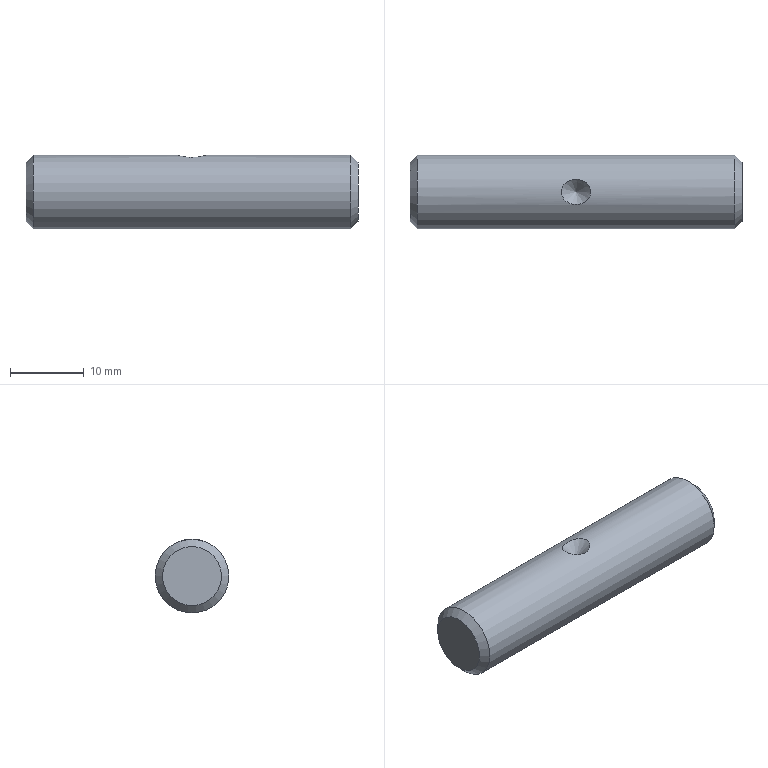Part | NX | features DATUM_CSYS 4, SKETCH 3, SWP104 2 | 1 solid | 6 faces | box 45 x 10 x 10 mm | volume 3498 mm3 | cone 3 | plane 2 | cylinder 1 | commonest cylinder face diameters 10 x1
STEP:
#1=CARTESIAN_POINT('',(-22.5,4.,0.));
#2=VERTEX_POINT('',#1);
#3=CARTESIAN_POINT('',(-22.5,0.,0.));
#4=DIRECTION('',(1.,0.,0.));
#5=DIRECTION('',(0.,1.,0.));
#6=AXIS2_PLACEMENT_3D('',#3,#4,#5);
#7=CIRCLE('',#6,4.);
#8=EDGE_CURVE('',#2,#2,#7,.T.);
#9=ORIENTED_EDGE('',*,*,#8,.T.);
#10=EDGE_LOOP('',(#9));
#11=FACE_BOUND('',#10,.T.);
#12=CARTESIAN_POINT('',(-21.5,5.,0.));
#13=VERTEX_POINT('',#12);
#14=CARTESIAN_POINT('',(-21.5,0.,0.));
#15=DIRECTION('',(1.,0.,0.));
#16=DIRECTION('',(0.,1.,0.));
#17=AXIS2_PLACEMENT_3D('',#14,#15,#16);
#18=CIRCLE('',#17,5.);
#19=EDGE_CURVE('',#13,#13,#18,.T.);
#20=ORIENTED_EDGE('',*,*,#19,.F.);
#21=EDGE_LOOP('',(#20));
#22=FACE_BOUND('',#21,.T.);
#23=CARTESIAN_POINT('',(-21.5,0.,0.));
#24=DIRECTION('',(1.,0.,0.));
#25=DIRECTION('',(0.,1.,0.));
#26=AXIS2_PLACEMENT_3D('',#23,#24,#25);
#27=CONICAL_SURFACE('',#26,5.,0.7854);
#28=ADVANCED_FACE('',(#11,#22),#27,.T.);
#29=ORIENTED_EDGE('',*,*,#8,.F.);
#30=EDGE_LOOP('',(#29));
#31=FACE_BOUND('',#30,.T.);
#32=CARTESIAN_POINT('',(-22.5,4.,0.));
#33=DIRECTION('',(-1.,0.,0.));
#34=DIRECTION('',(0.,-1.,0.));
#35=AXIS2_PLACEMENT_3D('',#32,#33,#34);
#36=PLANE('',#35);
#37=ADVANCED_FACE('',(#31),#36,.T.);
#38=CARTESIAN_POINT('',(22.5,4.,0.));
#39=VERTEX_POINT('',#38);
#40=CARTESIAN_POINT('',(22.5,0.,0.));
#41=DIRECTION('',(1.,0.,0.));
#42=DIRECTION('',(0.,1.,0.));
#43=AXIS2_PLACEMENT_3D('',#40,#41,#42);
#44=CIRCLE('',#43,4.);
#45=EDGE_CURVE('',#39,#39,#44,.T.);
#46=ORIENTED_EDGE('',*,*,#45,.T.);
#47=EDGE_LOOP('',(#46));
#48=FACE_BOUND('',#47,.T.);
#49=CARTESIAN_POINT('',(22.5,0.,0.));
#50=DIRECTION('',(1.,0.,0.));
#51=DIRECTION('',(0.,1.,0.));
#52=AXIS2_PLACEMENT_3D('',#49,#50,#51);
#53=PLANE('',#52);
#54=ADVANCED_FACE('',(#48),#53,.T.);
#55=CARTESIAN_POINT('',(21.5,5.,0.));
#56=VERTEX_POINT('',#55);
#57=CARTESIAN_POINT('',(21.5,0.,0.));
#58=DIRECTION('',(1.,0.,0.));
#59=DIRECTION('',(0.,1.,0.));
#60=AXIS2_PLACEMENT_3D('',#57,#58,#59);
#61=CIRCLE('',#60,5.);
#62=EDGE_CURVE('',#56,#56,#61,.T.);
#63=ORIENTED_EDGE('',*,*,#62,.T.);
#64=EDGE_LOOP('',(#63));
#65=FACE_BOUND('',#64,.T.);
#66=ORIENTED_EDGE('',*,*,#45,.F.);
#67=EDGE_LOOP('',(#66));
#68=FACE_BOUND('',#67,.T.);
#69=CARTESIAN_POINT('',(22.5,0.,0.));
#70=DIRECTION('',(-1.,0.,0.));
#71=DIRECTION('',(0.,-1.,0.));
#72=AXIS2_PLACEMENT_3D('',#69,#70,#71);
#73=CONICAL_SURFACE('',#72,4.,0.7854);
#74=ADVANCED_FACE('',(#65,#68),#73,.T.);
#75=CARTESIAN_POINT('',(-1.627,-0.9847,4.902));
#76=VERTEX_POINT('',#75);
#77=CARTESIAN_POINT('',(-2.199,0.4568,5.059));
#78=CARTESIAN_POINT('',(-1.791,-1.137,4.926));
#79=CARTESIAN_POINT('',(-0.4,-1.817,4.651));
#80=CARTESIAN_POINT('',(1.101,-1.613,4.748));
#81=CARTESIAN_POINT('',(2.198,-0.4566,5.059));
#82=CARTESIAN_POINT('',(1.794,1.133,4.926));
#83=CARTESIAN_POINT('',(0.401,1.818,4.651));
#84=CARTESIAN_POINT('',(-1.101,1.612,4.748));
#85=CARTESIAN_POINT('',(-2.199,0.4568,5.059));
#86=CARTESIAN_POINT('',(-1.791,-1.137,4.926));
#87=CARTESIAN_POINT('',(-0.4,-1.817,4.651));
#88=B_SPLINE_CURVE_WITH_KNOTS('',3,(#77,#78,#79,#80,#81,#82,#83,#84,#85,#86,#87),.UNSPECIFIED.,.T.,.F.,(1,1,1,1,1,1,1,1,1,1,1,1,1,1,1),(-0.00438,-0.00292,-0.00146,0.,0.00146,0.00292,0.00438,0.00584,0.0073,0.00876,0.01022,0.01168,0.01314,0.0146,0.01606),.UNSPECIFIED.);
#89=EDGE_CURVE('',#76,#76,#88,.T.);
#90=ORIENTED_EDGE('',*,*,#89,.F.);
#91=EDGE_LOOP('',(#90));
#92=FACE_BOUND('',#91,.T.);
#93=ORIENTED_EDGE('',*,*,#19,.T.);
#94=EDGE_LOOP('',(#93));
#95=FACE_BOUND('',#94,.T.);
#96=ORIENTED_EDGE('',*,*,#62,.F.);
#97=EDGE_LOOP('',(#96));
#98=FACE_BOUND('',#97,.T.);
#99=CARTESIAN_POINT('',(0.,0.,0.));
#100=DIRECTION('',(1.,0.,0.));
#101=DIRECTION('',(0.,1.,0.));
#102=AXIS2_PLACEMENT_3D('',#99,#100,#101);
#103=CYLINDRICAL_SURFACE('',#102,5.);
#104=ADVANCED_FACE('',(#92,#95,#98),#103,.T.);
#105=ORIENTED_EDGE('',*,*,#89,.T.);
#106=EDGE_LOOP('',(#105));
#107=FACE_BOUND('',#106,.T.);
#108=CARTESIAN_POINT('',(0.,0.,3.));
#109=VERTEX_POINT('',#108);
#110=VERTEX_LOOP('',#109);
#111=FACE_BOUND('',#110,.T.);
#112=CARTESIAN_POINT('',(0.,0.,3.));
#113=DIRECTION('',(0.,0.,1.));
#114=DIRECTION('',(1.,0.,0.));
#115=AXIS2_PLACEMENT_3D('',#112,#113,#114);
#116=CONICAL_SURFACE('',#115,0.,0.7854);
#117=ADVANCED_FACE('',(#107,#111),#116,.F.);
#118=CLOSED_SHELL('',(#28,#37,#54,#74,#104,#117));
#119=MANIFOLD_SOLID_BREP('',#118);
#120=(LENGTH_UNIT()NAMED_UNIT(*)SI_UNIT(.MILLI.,.METRE.));
#121=UNCERTAINTY_MEASURE_WITH_UNIT(LENGTH_MEASURE(0.0508),#120,'','');
#122=(NAMED_UNIT(*)PLANE_ANGLE_UNIT()SI_UNIT($,.RADIAN.));
#123=(NAMED_UNIT(*)SI_UNIT($,.STERADIAN.)SOLID_ANGLE_UNIT());
#124=(GEOMETRIC_REPRESENTATION_CONTEXT(3)GLOBAL_UNCERTAINTY_ASSIGNED_CONTEXT((#121))GLOBAL_UNIT_ASSIGNED_CONTEXT((#120,#122,#123))REPRESENTATION_CONTEXT('',''));
#125=ADVANCED_BREP_SHAPE_REPRESENTATION('',(#119),#124);